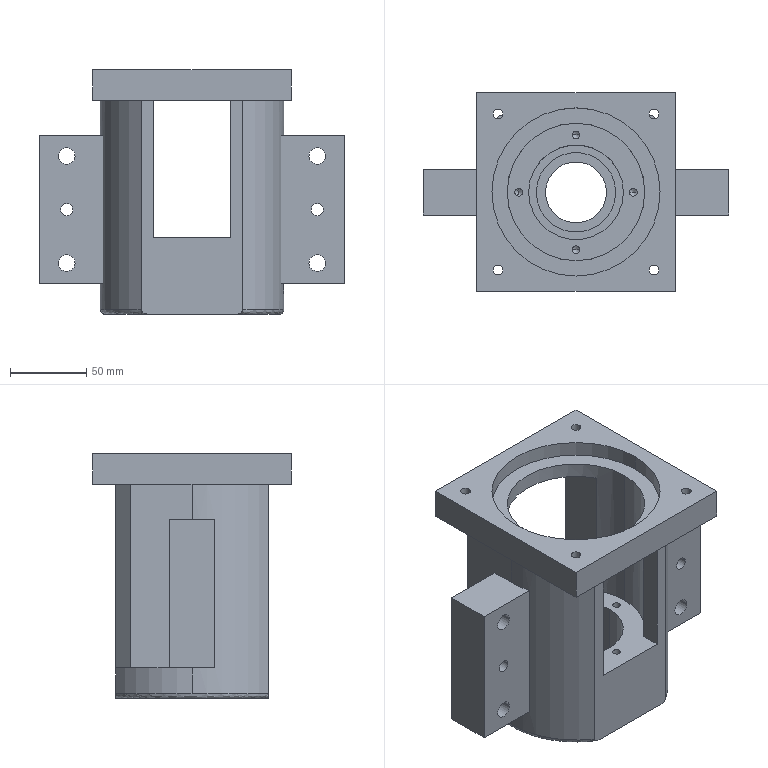Part | STEP file | 45L X-Direction Motor Mount | 1 solid | 100 faces | box 200 x 130 x 160 mm | volume 1107999 mm3 | cylinder 51 | plane 38 | cone 8 | spline 3 | commonest cylinder face diameters 5 x8 6.5 x8 11 x8 17 x8 8 x4 52 x4